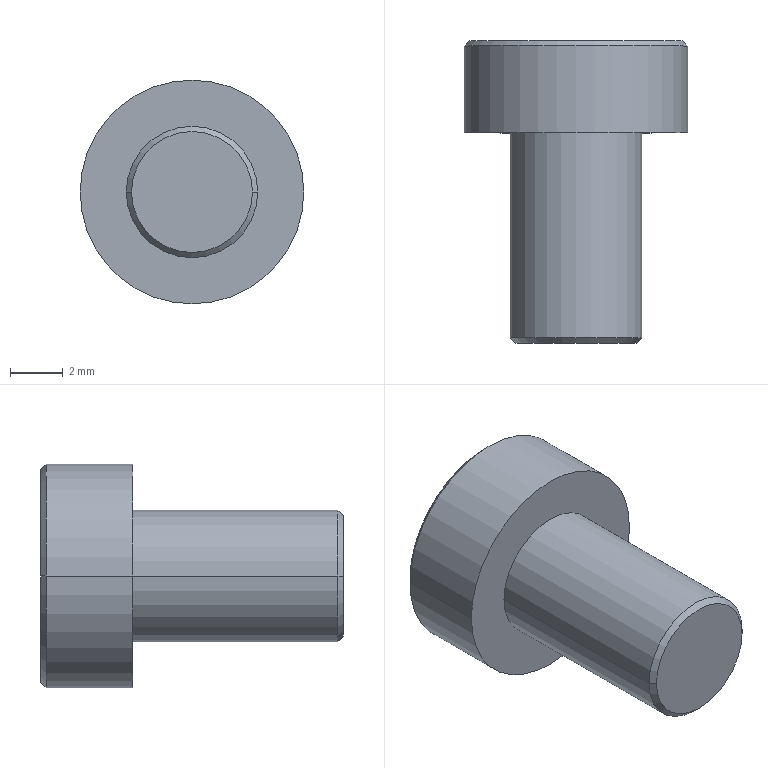Part | SolidWorks | features Chamfer 1, ICE 1, MoveCopyBody 1, Revolution 1 | 1 solid | 25 faces | box 8.5 x 11.5 x 8.5 mm | volume 331.771 mm3 | plane 15 | cone 6 | cylinder 4 | commonest cylinder face diameters 5 x2 8.5 x2
STEP:
#1=CARTESIAN_POINT('',(0.,6.434,0.));
#2=VERTEX_POINT('',#1);
#3=CARTESIAN_POINT('',(1.5,7.3,0.));
#4=VERTEX_POINT('',#3);
#5=CARTESIAN_POINT('',(0.,6.434,0.));
#6=DIRECTION('',(0.866,0.5,0.));
#7=VECTOR('',#6,1000.);
#8=LINE('',#5,#7);
#9=EDGE_CURVE('',#2,#4,#8,.T.);
#10=ORIENTED_EDGE('',*,*,#9,.F.);
#11=CARTESIAN_POINT('',(-1.5,7.3,0.));
#12=VERTEX_POINT('',#11);
#13=CARTESIAN_POINT('',(0.,6.434,0.));
#14=DIRECTION('',(-0.866,0.5,0.));
#15=VECTOR('',#14,1000.);
#16=LINE('',#13,#15);
#17=EDGE_CURVE('',#2,#12,#16,.T.);
#18=ORIENTED_EDGE('',*,*,#17,.T.);
#19=CARTESIAN_POINT('',(-1.299,7.3,0.75));
#20=VERTEX_POINT('',#19);
#21=CARTESIAN_POINT('',(0.,7.3,0.));
#22=DIRECTION('',(0.,1.,0.));
#23=DIRECTION('',(1.,0.,0.));
#24=AXIS2_PLACEMENT_3D('',#21,#22,#23);
#25=CIRCLE('',#24,1.5);
#26=EDGE_CURVE('',#12,#20,#25,.T.);
#27=ORIENTED_EDGE('',*,*,#26,.T.);
#28=CARTESIAN_POINT('',(0.,7.3,1.5));
#29=VERTEX_POINT('',#28);
#30=CARTESIAN_POINT('',(0.,7.3,0.));
#31=DIRECTION('',(0.,1.,0.));
#32=DIRECTION('',(1.,0.,0.));
#33=AXIS2_PLACEMENT_3D('',#30,#31,#32);
#34=CIRCLE('',#33,1.5);
#35=EDGE_CURVE('',#20,#29,#34,.T.);
#36=ORIENTED_EDGE('',*,*,#35,.T.);
#37=CARTESIAN_POINT('',(1.299,7.3,0.75));
#38=VERTEX_POINT('',#37);
#39=CARTESIAN_POINT('',(0.,7.3,0.));
#40=DIRECTION('',(0.,1.,0.));
#41=DIRECTION('',(1.,0.,0.));
#42=AXIS2_PLACEMENT_3D('',#39,#40,#41);
#43=CIRCLE('',#42,1.5);
#44=EDGE_CURVE('',#29,#38,#43,.T.);
#45=ORIENTED_EDGE('',*,*,#44,.T.);
#46=CARTESIAN_POINT('',(0.,7.3,0.));
#47=DIRECTION('',(0.,1.,0.));
#48=DIRECTION('',(1.,0.,0.));
#49=AXIS2_PLACEMENT_3D('',#46,#47,#48);
#50=CIRCLE('',#49,1.5);
#51=EDGE_CURVE('',#38,#4,#50,.T.);
#52=ORIENTED_EDGE('',*,*,#51,.T.);
#53=EDGE_LOOP('',(#10,#18,#27,#36,#45,#52));
#54=FACE_OUTER_BOUND('',#53,.T.);
#55=CARTESIAN_POINT('',(0.,1006.434,0.));
#56=DIRECTION('',(0.,1.,0.));
#57=DIRECTION('',(1.,0.,0.));
#58=AXIS2_PLACEMENT_3D('',#55,#56,#57);
#59=CONICAL_SURFACE('',#58,1732.051,1.047);
#60=ADVANCED_FACE('',(#54),#59,.F.);
#61=CARTESIAN_POINT('',(-2.3,-1.5,0.));
#62=VERTEX_POINT('',#61);
#63=CARTESIAN_POINT('',(2.3,-1.5,0.));
#64=VERTEX_POINT('',#63);
#65=CARTESIAN_POINT('',(0.,-1.5,0.));
#66=DIRECTION('',(0.,-1.,0.));
#67=DIRECTION('',(-1.,0.,0.));
#68=AXIS2_PLACEMENT_3D('',#65,#66,#67);
#69=CIRCLE('',#68,2.3);
#70=EDGE_CURVE('',#62,#64,#69,.T.);
#71=ORIENTED_EDGE('',*,*,#70,.F.);
#72=CARTESIAN_POINT('',(-2.5,-1.3,0.));
#73=VERTEX_POINT('',#72);
#74=CARTESIAN_POINT('',(-2.5,-1.3,0.));
#75=DIRECTION('',(-0.7071,0.7071,0.));
#76=VECTOR('',#75,1000.);
#77=LINE('',#74,#76);
#78=EDGE_CURVE('',#62,#73,#77,.T.);
#79=ORIENTED_EDGE('',*,*,#78,.T.);
#80=CARTESIAN_POINT('',(2.5,-1.3,0.));
#81=VERTEX_POINT('',#80);
#82=CARTESIAN_POINT('',(0.,-1.3,0.));
#83=DIRECTION('',(0.,1.,0.));
#84=DIRECTION('',(-1.,0.,0.));
#85=AXIS2_PLACEMENT_3D('',#82,#83,#84);
#86=CIRCLE('',#85,2.5);
#87=EDGE_CURVE('',#81,#73,#86,.T.);
#88=ORIENTED_EDGE('',*,*,#87,.F.);
#89=CARTESIAN_POINT('',(2.5,-1.3,0.));
#90=DIRECTION('',(0.7071,0.7071,0.));
#91=VECTOR('',#90,1000.);
#92=LINE('',#89,#91);
#93=EDGE_CURVE('',#64,#81,#92,.T.);
#94=ORIENTED_EDGE('',*,*,#93,.F.);
#95=EDGE_LOOP('',(#71,#79,#88,#94));
#96=FACE_OUTER_BOUND('',#95,.T.);
#97=CARTESIAN_POINT('',(0.,-1.3,0.));
#98=DIRECTION('',(0.,1.,0.));
#99=DIRECTION('',(1.,0.,0.));
#100=AXIS2_PLACEMENT_3D('',#97,#98,#99);
#101=CONICAL_SURFACE('',#100,2.5,0.7854);
#102=ADVANCED_FACE('',(#96),#101,.T.);
#103=CARTESIAN_POINT('',(4.05,10.,0.));
#104=VERTEX_POINT('',#103);
#105=CARTESIAN_POINT('',(-4.05,10.,0.));
#106=VERTEX_POINT('',#105);
#107=CARTESIAN_POINT('',(0.,10.,0.));
#108=DIRECTION('',(0.,1.,0.));
#109=DIRECTION('',(1.,0.,0.));
#110=AXIS2_PLACEMENT_3D('',#107,#108,#109);
#111=CIRCLE('',#110,4.05);
#112=EDGE_CURVE('',#104,#106,#111,.T.);
#113=ORIENTED_EDGE('',*,*,#112,.F.);
#114=CARTESIAN_POINT('',(4.25,9.8,0.));
#115=VERTEX_POINT('',#114);
#116=CARTESIAN_POINT('',(4.05,10.,0.));
#117=DIRECTION('',(0.7071,-0.7071,0.));
#118=VECTOR('',#117,1000.);
#119=LINE('',#116,#118);
#120=EDGE_CURVE('',#104,#115,#119,.T.);
#121=ORIENTED_EDGE('',*,*,#120,.T.);
#122=CARTESIAN_POINT('',(-4.25,9.8,0.));
#123=VERTEX_POINT('',#122);
#124=CARTESIAN_POINT('',(0.,9.8,0.));
#125=DIRECTION('',(0.,-1.,0.));
#126=DIRECTION('',(1.,0.,0.));
#127=AXIS2_PLACEMENT_3D('',#124,#125,#126);
#128=CIRCLE('',#127,4.25);
#129=EDGE_CURVE('',#123,#115,#128,.T.);
#130=ORIENTED_EDGE('',*,*,#129,.F.);
#131=CARTESIAN_POINT('',(-4.05,10.,0.));
#132=DIRECTION('',(-0.7071,-0.7071,0.));
#133=VECTOR('',#132,1000.);
#134=LINE('',#131,#133);
#135=EDGE_CURVE('',#106,#123,#134,.T.);
#136=ORIENTED_EDGE('',*,*,#135,.F.);
#137=EDGE_LOOP('',(#113,#121,#130,#136));
#138=FACE_OUTER_BOUND('',#137,.T.);
#139=CARTESIAN_POINT('',(0.,10.,0.));
#140=DIRECTION('',(0.,-1.,0.));
#141=DIRECTION('',(-1.,0.,0.));
#142=AXIS2_PLACEMENT_3D('',#139,#140,#141);
#143=CONICAL_SURFACE('',#142,4.05,0.7854);
#144=ADVANCED_FACE('',(#138),#143,.T.);
#145=CARTESIAN_POINT('',(4.25,6.5,0.));
#146=VERTEX_POINT('',#145);
#147=CARTESIAN_POINT('',(-4.25,6.5,0.));
#148=VERTEX_POINT('',#147);
#149=CARTESIAN_POINT('',(0.,6.5,0.));
#150=DIRECTION('',(0.,1.,0.));
#151=DIRECTION('',(1.,0.,0.));
#152=AXIS2_PLACEMENT_3D('',#149,#150,#151);
#153=CIRCLE('',#152,4.25);
#154=EDGE_CURVE('',#146,#148,#153,.T.);
#155=ORIENTED_EDGE('',*,*,#154,.T.);
#156=CARTESIAN_POINT('',(-4.25,6.434,0.));
#157=DIRECTION('',(0.,1.,0.));
#158=VECTOR('',#157,1000.);
#159=LINE('',#156,#158);
#160=EDGE_CURVE('',#148,#123,#159,.T.);
#161=ORIENTED_EDGE('',*,*,#160,.T.);
#162=ORIENTED_EDGE('',*,*,#129,.T.);
#163=CARTESIAN_POINT('',(4.25,6.434,0.));
#164=DIRECTION('',(0.,1.,0.));
#165=VECTOR('',#164,1000.);
#166=LINE('',#163,#165);
#167=EDGE_CURVE('',#146,#115,#166,.T.);
#168=ORIENTED_EDGE('',*,*,#167,.F.);
#169=EDGE_LOOP('',(#155,#161,#162,#168));
#170=FACE_OUTER_BOUND('',#169,.T.);
#171=CARTESIAN_POINT('',(0.,6.434,0.));
#172=DIRECTION('',(0.,1.,0.));
#173=DIRECTION('',(1.,0.,0.));
#174=AXIS2_PLACEMENT_3D('',#171,#172,#173);
#175=CYLINDRICAL_SURFACE('',#174,4.25);
#176=ADVANCED_FACE('',(#170),#175,.T.);
#177=ORIENTED_EDGE('',*,*,#87,.T.);
#178=CARTESIAN_POINT('',(-2.5,6.5,0.));
#179=VERTEX_POINT('',#178);
#180=CARTESIAN_POINT('',(-2.5,6.434,0.));
#181=DIRECTION('',(0.,1.,0.));
#182=VECTOR('',#181,1000.);
#183=LINE('',#180,#182);
#184=EDGE_CURVE('',#73,#179,#183,.T.);
#185=ORIENTED_EDGE('',*,*,#184,.T.);
#186=CARTESIAN_POINT('',(2.5,6.5,0.));
#187=VERTEX_POINT('',#186);
#188=CARTESIAN_POINT('',(0.,6.5,0.));
#189=DIRECTION('',(0.,1.,0.));
#190=DIRECTION('',(1.,0.,0.));
#191=AXIS2_PLACEMENT_3D('',#188,#189,#190);
#192=CIRCLE('',#191,2.5);
#193=EDGE_CURVE('',#187,#179,#192,.T.);
#194=ORIENTED_EDGE('',*,*,#193,.F.);
#195=CARTESIAN_POINT('',(2.5,6.434,0.));
#196=DIRECTION('',(0.,1.,0.));
#197=VECTOR('',#196,1000.);
#198=LINE('',#195,#197);
#199=EDGE_CURVE('',#81,#187,#198,.T.);
#200=ORIENTED_EDGE('',*,*,#199,.F.);
#201=EDGE_LOOP('',(#177,#185,#194,#200));
#202=FACE_OUTER_BOUND('',#201,.T.);
#203=CARTESIAN_POINT('',(0.,6.434,0.));
#204=DIRECTION('',(0.,1.,0.));
#205=DIRECTION('',(1.,0.,0.));
#206=AXIS2_PLACEMENT_3D('',#203,#204,#205);
#207=CYLINDRICAL_SURFACE('',#206,2.5);
#208=ADVANCED_FACE('',(#202),#207,.T.);
#209=CARTESIAN_POINT('',(0.866,10.,1.5));
#210=VERTEX_POINT('',#209);
#211=CARTESIAN_POINT('',(1.732,10.,0.));
#212=VERTEX_POINT('',#211);
#213=CARTESIAN_POINT('',(0.866,10.,1.5));
#214=DIRECTION('',(0.5,0.,-0.866));
#215=VECTOR('',#214,1000.);
#216=LINE('',#213,#215);
#217=EDGE_CURVE('',#210,#212,#216,.T.);
#218=ORIENTED_EDGE('',*,*,#217,.F.);
#219=CARTESIAN_POINT('',(-0.866,10.,1.5));
#220=VERTEX_POINT('',#219);
#221=CARTESIAN_POINT('',(-0.866,10.,1.5));
#222=DIRECTION('',(1.,0.,0.));
#223=VECTOR('',#222,1000.);
#224=LINE('',#221,#223);
#225=EDGE_CURVE('',#220,#210,#224,.T.);
#226=ORIENTED_EDGE('',*,*,#225,.F.);
#227=CARTESIAN_POINT('',(-1.732,10.,0.));
#228=VERTEX_POINT('',#227);
#229=CARTESIAN_POINT('',(-1.732,10.,0.));
#230=DIRECTION('',(0.5,0.,0.866));
#231=VECTOR('',#230,1000.);
#232=LINE('',#229,#231);
#233=EDGE_CURVE('',#228,#220,#232,.T.);
#234=ORIENTED_EDGE('',*,*,#233,.F.);
#235=CARTESIAN_POINT('',(-0.866,10.,-1.5));
#236=VERTEX_POINT('',#235);
#237=CARTESIAN_POINT('',(-0.866,10.,-1.5));
#238=DIRECTION('',(-0.5,0.,0.866));
#239=VECTOR('',#238,1000.);
#240=LINE('',#237,#239);
#241=EDGE_CURVE('',#236,#228,#240,.T.);
#242=ORIENTED_EDGE('',*,*,#241,.F.);
#243=CARTESIAN_POINT('',(0.866,10.,-1.5));
#244=VERTEX_POINT('',#243);
#245=CARTESIAN_POINT('',(0.866,10.,-1.5));
#246=DIRECTION('',(-1.,0.,0.));
#247=VECTOR('',#246,1000.);
#248=LINE('',#245,#247);
#249=EDGE_CURVE('',#244,#236,#248,.T.);
#250=ORIENTED_EDGE('',*,*,#249,.F.);
#251=CARTESIAN_POINT('',(1.732,10.,0.));
#252=DIRECTION('',(-0.5,0.,-0.866));
#253=VECTOR('',#252,1000.);
#254=LINE('',#251,#253);
#255=EDGE_CURVE('',#212,#244,#254,.T.);
#256=ORIENTED_EDGE('',*,*,#255,.F.);
#257=EDGE_LOOP('',(#218,#226,#234,#242,#250,#256));
#258=FACE_BOUND('',#257,.T.);
#259=CARTESIAN_POINT('',(0.,10.,0.));
#260=DIRECTION('',(0.,1.,0.));
#261=DIRECTION('',(1.,0.,0.));
#262=AXIS2_PLACEMENT_3D('',#259,#260,#261);
#263=CIRCLE('',#262,4.05);
#264=EDGE_CURVE('',#106,#104,#263,.T.);
#265=ORIENTED_EDGE('',*,*,#264,.T.);
#266=ORIENTED_EDGE('',*,*,#112,.T.);
#267=EDGE_LOOP('',(#265,#266));
#268=FACE_OUTER_BOUND('',#267,.T.);
#269=CARTESIAN_POINT('',(-4.25,10.,0.));
#270=DIRECTION('',(0.,1.,0.));
#271=DIRECTION('',(1.,0.,0.));
#272=AXIS2_PLACEMENT_3D('',#269,#270,#271);
#273=PLANE('',#272);
#274=ADVANCED_FACE('',(#258,#268),#273,.T.);
#275=CARTESIAN_POINT('',(0.,-1.5,0.));
#276=DIRECTION('',(0.,-1.,0.));
#277=DIRECTION('',(-1.,0.,0.));
#278=AXIS2_PLACEMENT_3D('',#275,#276,#277);
#279=CIRCLE('',#278,2.3);
#280=EDGE_CURVE('',#64,#62,#279,.T.);
#281=ORIENTED_EDGE('',*,*,#280,.T.);
#282=ORIENTED_EDGE('',*,*,#70,.T.);
#283=EDGE_LOOP('',(#281,#282));
#284=FACE_OUTER_BOUND('',#283,.T.);
#285=CARTESIAN_POINT('',(-2.5,-1.5,0.));
#286=DIRECTION('',(0.,-1.,0.));
#287=DIRECTION('',(-1.,0.,0.));
#288=AXIS2_PLACEMENT_3D('',#285,#286,#287);
#289=PLANE('',#288);
#290=ADVANCED_FACE('',(#284),#289,.T.);
#291=ORIENTED_EDGE('',*,*,#184,.F.);
#292=CARTESIAN_POINT('',(0.,-1.3,0.));
#293=DIRECTION('',(0.,1.,0.));
#294=DIRECTION('',(-1.,0.,0.));
#295=AXIS2_PLACEMENT_3D('',#292,#293,#294);
#296=CIRCLE('',#295,2.5);
#297=EDGE_CURVE('',#73,#81,#296,.T.);
#298=ORIENTED_EDGE('',*,*,#297,.T.);
#299=ORIENTED_EDGE('',*,*,#199,.T.);
#300=CARTESIAN_POINT('',(0.,6.5,0.));
#301=DIRECTION('',(0.,1.,0.));
#302=DIRECTION('',(1.,0.,0.));
#303=AXIS2_PLACEMENT_3D('',#300,#301,#302);
#304=CIRCLE('',#303,2.5);
#305=EDGE_CURVE('',#179,#187,#304,.T.);
#306=ORIENTED_EDGE('',*,*,#305,.F.);
#307=EDGE_LOOP('',(#291,#298,#299,#306));
#308=FACE_OUTER_BOUND('',#307,.T.);
#309=CARTESIAN_POINT('',(0.,6.434,0.));
#310=DIRECTION('',(0.,1.,0.));
#311=DIRECTION('',(1.,0.,0.));
#312=AXIS2_PLACEMENT_3D('',#309,#310,#311);
#313=CYLINDRICAL_SURFACE('',#312,2.5);
#314=ADVANCED_FACE('',(#308),#313,.T.);
#315=ORIENTED_EDGE('',*,*,#193,.T.);
#316=ORIENTED_EDGE('',*,*,#305,.T.);
#317=EDGE_LOOP('',(#315,#316));
#318=FACE_BOUND('',#317,.T.);
#319=ORIENTED_EDGE('',*,*,#154,.F.);
#320=CARTESIAN_POINT('',(0.,6.5,0.));
#321=DIRECTION('',(0.,1.,0.));
#322=DIRECTION('',(1.,0.,0.));
#323=AXIS2_PLACEMENT_3D('',#320,#321,#322);
#324=CIRCLE('',#323,4.25);
#325=EDGE_CURVE('',#148,#146,#324,.T.);
#326=ORIENTED_EDGE('',*,*,#325,.F.);
#327=EDGE_LOOP('',(#319,#326));
#328=FACE_OUTER_BOUND('',#327,.T.);
#329=CARTESIAN_POINT('',(-2.5,6.5,0.));
#330=DIRECTION('',(0.,-1.,0.));
#331=DIRECTION('',(-1.,0.,0.));
#332=AXIS2_PLACEMENT_3D('',#329,#330,#331);
#333=PLANE('',#332);
#334=ADVANCED_FACE('',(#318,#328),#333,.T.);
#335=ORIENTED_EDGE('',*,*,#160,.F.);
#336=ORIENTED_EDGE('',*,*,#325,.T.);
#337=ORIENTED_EDGE('',*,*,#167,.T.);
#338=CARTESIAN_POINT('',(0.,9.8,0.));
#339=DIRECTION('',(0.,-1.,0.));
#340=DIRECTION('',(1.,0.,0.));
#341=AXIS2_PLACEMENT_3D('',#338,#339,#340);
#342=CIRCLE('',#341,4.25);
#343=EDGE_CURVE('',#115,#123,#342,.T.);
#344=ORIENTED_EDGE('',*,*,#343,.T.);
#345=EDGE_LOOP('',(#335,#336,#337,#344));
#346=FACE_OUTER_BOUND('',#345,.T.);
#347=CARTESIAN_POINT('',(0.,6.434,0.));
#348=DIRECTION('',(0.,1.,0.));
#349=DIRECTION('',(1.,0.,0.));
#350=AXIS2_PLACEMENT_3D('',#347,#348,#349);
#351=CYLINDRICAL_SURFACE('',#350,4.25);
#352=ADVANCED_FACE('',(#346),#351,.T.);
#353=ORIENTED_EDGE('',*,*,#120,.F.);
#354=ORIENTED_EDGE('',*,*,#264,.F.);
#355=ORIENTED_EDGE('',*,*,#135,.T.);
#356=ORIENTED_EDGE('',*,*,#343,.F.);
#357=EDGE_LOOP('',(#353,#354,#355,#356));
#358=FACE_OUTER_BOUND('',#357,.T.);
#359=CARTESIAN_POINT('',(0.,10.,0.));
#360=DIRECTION('',(0.,-1.,0.));
#361=DIRECTION('',(-1.,0.,0.));
#362=AXIS2_PLACEMENT_3D('',#359,#360,#361);
#363=CONICAL_SURFACE('',#362,4.05,0.7854);
#364=ADVANCED_FACE('',(#358),#363,.T.);
#365=ORIENTED_EDGE('',*,*,#78,.F.);
#366=ORIENTED_EDGE('',*,*,#280,.F.);
#367=ORIENTED_EDGE('',*,*,#93,.T.);
#368=ORIENTED_EDGE('',*,*,#297,.F.);
#369=EDGE_LOOP('',(#365,#366,#367,#368));
#370=FACE_OUTER_BOUND('',#369,.T.);
#371=CARTESIAN_POINT('',(0.,-1.3,0.));
#372=DIRECTION('',(0.,1.,0.));
#373=DIRECTION('',(1.,0.,0.));
#374=AXIS2_PLACEMENT_3D('',#371,#372,#373);
#375=CONICAL_SURFACE('',#374,2.5,0.7854);
#376=ADVANCED_FACE('',(#370),#375,.T.);
#377=CARTESIAN_POINT('',(0.866,7.3,-1.5));
#378=VERTEX_POINT('',#377);
#379=CARTESIAN_POINT('',(0.,7.3,-1.5));
#380=VERTEX_POINT('',#379);
#381=CARTESIAN_POINT('',(0.866,7.3,-1.5));
#382=DIRECTION('',(-1.,0.,0.));
#383=VECTOR('',#382,1000.);
#384=LINE('',#381,#383);
#385=EDGE_CURVE('',#378,#380,#384,.T.);
#386=ORIENTED_EDGE('',*,*,#385,.F.);
#387=CARTESIAN_POINT('',(0.866,7.3,-1.5));
#388=DIRECTION('',(0.,1.,0.));
#389=VECTOR('',#388,1000.);
#390=LINE('',#387,#389);
#391=EDGE_CURVE('',#378,#244,#390,.T.);
#392=ORIENTED_EDGE('',*,*,#391,.T.);
#393=ORIENTED_EDGE('',*,*,#249,.T.);
#394=CARTESIAN_POINT('',(-0.866,7.3,-1.5));
#395=VERTEX_POINT('',#394);
#396=CARTESIAN_POINT('',(-0.866,7.3,-1.5));
#397=DIRECTION('',(0.,1.,0.));
#398=VECTOR('',#397,1000.);
#399=LINE('',#396,#398);
#400=EDGE_CURVE('',#395,#236,#399,.T.);
#401=ORIENTED_EDGE('',*,*,#400,.F.);
#402=CARTESIAN_POINT('',(0.866,7.3,-1.5));
#403=DIRECTION('',(-1.,0.,0.));
#404=VECTOR('',#403,1000.);
#405=LINE('',#402,#404);
#406=EDGE_CURVE('',#380,#395,#405,.T.);
#407=ORIENTED_EDGE('',*,*,#406,.F.);
#408=EDGE_LOOP('',(#386,#392,#393,#401,#407));
#409=FACE_OUTER_BOUND('',#408,.T.);
#410=CARTESIAN_POINT('',(0.866,7.3,-1.5));
#411=DIRECTION('',(0.,0.,-1.));
#412=DIRECTION('',(1.,0.,0.));
#413=AXIS2_PLACEMENT_3D('',#410,#411,#412);
#414=PLANE('',#413);
#415=ADVANCED_FACE('',(#409),#414,.F.);
#416=CARTESIAN_POINT('',(1.732,7.3,0.));
#417=VERTEX_POINT('',#416);
#418=CARTESIAN_POINT('',(1.299,7.3,-0.75));
#419=VERTEX_POINT('',#418);
#420=CARTESIAN_POINT('',(1.732,7.3,0.));
#421=DIRECTION('',(-0.5,0.,-0.866));
#422=VECTOR('',#421,1000.);
#423=LINE('',#420,#422);
#424=EDGE_CURVE('',#417,#419,#423,.T.);
#425=ORIENTED_EDGE('',*,*,#424,.F.);
#426=CARTESIAN_POINT('',(1.732,7.3,0.));
#427=DIRECTION('',(0.,1.,0.));
#428=VECTOR('',#427,1000.);
#429=LINE('',#426,#428);
#430=EDGE_CURVE('',#417,#212,#429,.T.);
#431=ORIENTED_EDGE('',*,*,#430,.T.);
#432=ORIENTED_EDGE('',*,*,#255,.T.);
#433=ORIENTED_EDGE('',*,*,#391,.F.);
#434=CARTESIAN_POINT('',(1.732,7.3,0.));
#435=DIRECTION('',(-0.5,0.,-0.866));
#436=VECTOR('',#435,1000.);
#437=LINE('',#434,#436);
#438=EDGE_CURVE('',#419,#378,#437,.T.);
#439=ORIENTED_EDGE('',*,*,#438,.F.);
#440=EDGE_LOOP('',(#425,#431,#432,#433,#439));
#441=FACE_OUTER_BOUND('',#440,.T.);
#442=CARTESIAN_POINT('',(1.732,7.3,0.));
#443=DIRECTION('',(0.866,0.,-0.5));
#444=DIRECTION('',(0.5,0.,0.866));
#445=AXIS2_PLACEMENT_3D('',#442,#443,#444);
#446=PLANE('',#445);
#447=ADVANCED_FACE('',(#441),#446,.F.);
#448=CARTESIAN_POINT('',(0.866,7.3,1.5));
#449=VERTEX_POINT('',#448);
#450=CARTESIAN_POINT('',(0.866,7.3,1.5));
#451=DIRECTION('',(0.5,0.,-0.866));
#452=VECTOR('',#451,1000.);
#453=LINE('',#450,#452);
#454=EDGE_CURVE('',#449,#38,#453,.T.);
#455=ORIENTED_EDGE('',*,*,#454,.F.);
#456=CARTESIAN_POINT('',(0.866,7.3,1.5));
#457=DIRECTION('',(0.,1.,0.));
#458=VECTOR('',#457,1000.);
#459=LINE('',#456,#458);
#460=EDGE_CURVE('',#449,#210,#459,.T.);
#461=ORIENTED_EDGE('',*,*,#460,.T.);
#462=ORIENTED_EDGE('',*,*,#217,.T.);
#463=ORIENTED_EDGE('',*,*,#430,.F.);
#464=CARTESIAN_POINT('',(0.866,7.3,1.5));
#465=DIRECTION('',(0.5,0.,-0.866));
#466=VECTOR('',#465,1000.);
#467=LINE('',#464,#466);
#468=EDGE_CURVE('',#38,#417,#467,.T.);
#469=ORIENTED_EDGE('',*,*,#468,.F.);
#470=EDGE_LOOP('',(#455,#461,#462,#463,#469));
#471=FACE_OUTER_BOUND('',#470,.T.);
#472=CARTESIAN_POINT('',(0.866,7.3,1.5));
#473=DIRECTION('',(0.866,0.,0.5));
#474=DIRECTION('',(-0.5,0.,0.866));
#475=AXIS2_PLACEMENT_3D('',#472,#473,#474);
#476=PLANE('',#475);
#477=ADVANCED_FACE('',(#471),#476,.F.);
#478=CARTESIAN_POINT('',(-0.866,7.3,1.5));
#479=VERTEX_POINT('',#478);
#480=CARTESIAN_POINT('',(-0.866,7.3,1.5));
#481=DIRECTION('',(1.,0.,0.));
#482=VECTOR('',#481,1000.);
#483=LINE('',#480,#482);
#484=EDGE_CURVE('',#479,#29,#483,.T.);
#485=ORIENTED_EDGE('',*,*,#484,.F.);
#486=CARTESIAN_POINT('',(-0.866,7.3,1.5));
#487=DIRECTION('',(0.,1.,0.));
#488=VECTOR('',#487,1000.);
#489=LINE('',#486,#488);
#490=EDGE_CURVE('',#479,#220,#489,.T.);
#491=ORIENTED_EDGE('',*,*,#490,.T.);
#492=ORIENTED_EDGE('',*,*,#225,.T.);
#493=ORIENTED_EDGE('',*,*,#460,.F.);
#494=CARTESIAN_POINT('',(-0.866,7.3,1.5));
#495=DIRECTION('',(1.,0.,0.));
#496=VECTOR('',#495,1000.);
#497=LINE('',#494,#496);
#498=EDGE_CURVE('',#29,#449,#497,.T.);
#499=ORIENTED_EDGE('',*,*,#498,.F.);
#500=EDGE_LOOP('',(#485,#491,#492,#493,#499));
#501=FACE_OUTER_BOUND('',#500,.T.);
#502=CARTESIAN_POINT('',(-0.866,7.3,1.5));
#503=DIRECTION('',(0.,0.,1.));
#504=DIRECTION('',(-1.,0.,0.));
#505=AXIS2_PLACEMENT_3D('',#502,#503,#504);
#506=PLANE('',#505);
#507=ADVANCED_FACE('',(#501),#506,.F.);
#508=CARTESIAN_POINT('',(-1.732,7.3,0.));
#509=VERTEX_POINT('',#508);
#510=CARTESIAN_POINT('',(-1.732,7.3,0.));
#511=DIRECTION('',(0.5,0.,0.866));
#512=VECTOR('',#511,1000.);
#513=LINE('',#510,#512);
#514=EDGE_CURVE('',#509,#20,#513,.T.);
#515=ORIENTED_EDGE('',*,*,#514,.F.);
#516=CARTESIAN_POINT('',(-1.732,7.3,0.));
#517=DIRECTION('',(0.,1.,0.));
#518=VECTOR('',#517,1000.);
#519=LINE('',#516,#518);
#520=EDGE_CURVE('',#509,#228,#519,.T.);
#521=ORIENTED_EDGE('',*,*,#520,.T.);
#522=ORIENTED_EDGE('',*,*,#233,.T.);
#523=ORIENTED_EDGE('',*,*,#490,.F.);
#524=CARTESIAN_POINT('',(-1.732,7.3,0.));
#525=DIRECTION('',(0.5,0.,0.866));
#526=VECTOR('',#525,1000.);
#527=LINE('',#524,#526);
#528=EDGE_CURVE('',#20,#479,#527,.T.);
#529=ORIENTED_EDGE('',*,*,#528,.F.);
#530=EDGE_LOOP('',(#515,#521,#522,#523,#529));
#531=FACE_OUTER_BOUND('',#530,.T.);
#532=CARTESIAN_POINT('',(-1.732,7.3,0.));
#533=DIRECTION('',(-0.866,0.,0.5));
#534=DIRECTION('',(-0.5,0.,-0.866));
#535=AXIS2_PLACEMENT_3D('',#532,#533,#534);
#536=PLANE('',#535);
#537=ADVANCED_FACE('',(#531),#536,.F.);
#538=CARTESIAN_POINT('',(-1.299,7.3,-0.75));
#539=VERTEX_POINT('',#538);
#540=CARTESIAN_POINT('',(-0.866,7.3,-1.5));
#541=DIRECTION('',(-0.5,0.,0.866));
#542=VECTOR('',#541,1000.);
#543=LINE('',#540,#542);
#544=EDGE_CURVE('',#395,#539,#543,.T.);
#545=ORIENTED_EDGE('',*,*,#544,.F.);
#546=ORIENTED_EDGE('',*,*,#400,.T.);
#547=ORIENTED_EDGE('',*,*,#241,.T.);
#548=ORIENTED_EDGE('',*,*,#520,.F.);
#549=CARTESIAN_POINT('',(-0.866,7.3,-1.5));
#550=DIRECTION('',(-0.5,0.,0.866));
#551=VECTOR('',#550,1000.);
#552=LINE('',#549,#551);
#553=EDGE_CURVE('',#539,#509,#552,.T.);
#554=ORIENTED_EDGE('',*,*,#553,.F.);
#555=EDGE_LOOP('',(#545,#546,#547,#548,#554));
#556=FACE_OUTER_BOUND('',#555,.T.);
#557=CARTESIAN_POINT('',(-0.866,7.3,-1.5));
#558=DIRECTION('',(-0.866,0.,-0.5));
#559=DIRECTION('',(0.5,0.,-0.866));
#560=AXIS2_PLACEMENT_3D('',#557,#558,#559);
#561=PLANE('',#560);
#562=ADVANCED_FACE('',(#556),#561,.F.);
#563=ORIENTED_EDGE('',*,*,#498,.T.);
#564=ORIENTED_EDGE('',*,*,#454,.T.);
#565=ORIENTED_EDGE('',*,*,#44,.F.);
#566=EDGE_LOOP('',(#563,#564,#565));
#567=FACE_OUTER_BOUND('',#566,.T.);
#568=CARTESIAN_POINT('',(-0.866,7.3,-1.5));
#569=DIRECTION('',(0.,1.,0.));
#570=DIRECTION('',(0.,0.,1.));
#571=AXIS2_PLACEMENT_3D('',#568,#569,#570);
#572=PLANE('',#571);
#573=ADVANCED_FACE('',(#567),#572,.T.);
#574=ORIENTED_EDGE('',*,*,#468,.T.);
#575=ORIENTED_EDGE('',*,*,#424,.T.);
#576=CARTESIAN_POINT('',(0.,7.3,0.));
#577=DIRECTION('',(0.,1.,0.));
#578=DIRECTION('',(1.,0.,0.));
#579=AXIS2_PLACEMENT_3D('',#576,#577,#578);
#580=CIRCLE('',#579,1.5);
#581=EDGE_CURVE('',#4,#419,#580,.T.);
#582=ORIENTED_EDGE('',*,*,#581,.F.);
#583=ORIENTED_EDGE('',*,*,#51,.F.);
#584=EDGE_LOOP('',(#574,#575,#582,#583));
#585=FACE_OUTER_BOUND('',#584,.T.);
#586=CARTESIAN_POINT('',(-0.866,7.3,-1.5));
#587=DIRECTION('',(0.,1.,0.));
#588=DIRECTION('',(0.,0.,1.));
#589=AXIS2_PLACEMENT_3D('',#586,#587,#588);
#590=PLANE('',#589);
#591=ADVANCED_FACE('',(#585),#590,.T.);
#592=ORIENTED_EDGE('',*,*,#438,.T.);
#593=ORIENTED_EDGE('',*,*,#385,.T.);
#594=CARTESIAN_POINT('',(0.,7.3,0.));
#595=DIRECTION('',(0.,1.,0.));
#596=DIRECTION('',(1.,0.,0.));
#597=AXIS2_PLACEMENT_3D('',#594,#595,#596);
#598=CIRCLE('',#597,1.5);
#599=EDGE_CURVE('',#419,#380,#598,.T.);
#600=ORIENTED_EDGE('',*,*,#599,.F.);
#601=EDGE_LOOP('',(#592,#593,#600));
#602=FACE_OUTER_BOUND('',#601,.T.);
#603=CARTESIAN_POINT('',(-0.866,7.3,-1.5));
#604=DIRECTION('',(0.,1.,0.));
#605=DIRECTION('',(0.,0.,1.));
#606=AXIS2_PLACEMENT_3D('',#603,#604,#605);
#607=PLANE('',#606);
#608=ADVANCED_FACE('',(#602),#607,.T.);
#609=ORIENTED_EDGE('',*,*,#406,.T.);
#610=ORIENTED_EDGE('',*,*,#544,.T.);
#611=CARTESIAN_POINT('',(0.,7.3,0.));
#612=DIRECTION('',(0.,1.,0.));
#613=DIRECTION('',(1.,0.,0.));
#614=AXIS2_PLACEMENT_3D('',#611,#612,#613);
#615=CIRCLE('',#614,1.5);
#616=EDGE_CURVE('',#380,#539,#615,.T.);
#617=ORIENTED_EDGE('',*,*,#616,.F.);
#618=EDGE_LOOP('',(#609,#610,#617));
#619=FACE_OUTER_BOUND('',#618,.T.);
#620=CARTESIAN_POINT('',(-0.866,7.3,-1.5));
#621=DIRECTION('',(0.,1.,0.));
#622=DIRECTION('',(0.,0.,1.));
#623=AXIS2_PLACEMENT_3D('',#620,#621,#622);
#624=PLANE('',#623);
#625=ADVANCED_FACE('',(#619),#624,.T.);
#626=ORIENTED_EDGE('',*,*,#553,.T.);
#627=ORIENTED_EDGE('',*,*,#514,.T.);
#628=ORIENTED_EDGE('',*,*,#26,.F.);
#629=CARTESIAN_POINT('',(0.,7.3,0.));
#630=DIRECTION('',(0.,1.,0.));
#631=DIRECTION('',(1.,0.,0.));
#632=AXIS2_PLACEMENT_3D('',#629,#630,#631);
#633=CIRCLE('',#632,1.5);
#634=EDGE_CURVE('',#539,#12,#633,.T.);
#635=ORIENTED_EDGE('',*,*,#634,.F.);
#636=EDGE_LOOP('',(#626,#627,#628,#635));
#637=FACE_OUTER_BOUND('',#636,.T.);
#638=CARTESIAN_POINT('',(-0.866,7.3,-1.5));
#639=DIRECTION('',(0.,1.,0.));
#640=DIRECTION('',(0.,0.,1.));
#641=AXIS2_PLACEMENT_3D('',#638,#639,#640);
#642=PLANE('',#641);
#643=ADVANCED_FACE('',(#637),#642,.T.);
#644=ORIENTED_EDGE('',*,*,#528,.T.);
#645=ORIENTED_EDGE('',*,*,#484,.T.);
#646=ORIENTED_EDGE('',*,*,#35,.F.);
#647=EDGE_LOOP('',(#644,#645,#646));
#648=FACE_OUTER_BOUND('',#647,.T.);
#649=CARTESIAN_POINT('',(-0.866,7.3,-1.5));
#650=DIRECTION('',(0.,1.,0.));
#651=DIRECTION('',(0.,0.,1.));
#652=AXIS2_PLACEMENT_3D('',#649,#650,#651);
#653=PLANE('',#652);
#654=ADVANCED_FACE('',(#648),#653,.T.);
#655=ORIENTED_EDGE('',*,*,#17,.F.);
#656=ORIENTED_EDGE('',*,*,#9,.T.);
#657=ORIENTED_EDGE('',*,*,#581,.T.);
#658=ORIENTED_EDGE('',*,*,#599,.T.);
#659=ORIENTED_EDGE('',*,*,#616,.T.);
#660=ORIENTED_EDGE('',*,*,#634,.T.);
#661=EDGE_LOOP('',(#655,#656,#657,#658,#659,#660));
#662=FACE_OUTER_BOUND('',#661,.T.);
#663=CARTESIAN_POINT('',(0.,1006.434,0.));
#664=DIRECTION('',(0.,1.,0.));
#665=DIRECTION('',(1.,0.,0.));
#666=AXIS2_PLACEMENT_3D('',#663,#664,#665);
#667=CONICAL_SURFACE('',#666,1732.051,1.047);
#668=ADVANCED_FACE('',(#662),#667,.F.);
#669=CLOSED_SHELL('',(#60,#102,#144,#176,#208,#274,#290,#314,#334,#352,#364,#376,#415,#447,#477,#507,#537,#562,#573,#591,#608,#625,#643,#654,#668));
#670=MANIFOLD_SOLID_BREP('',#669);
#671=CARTESIAN_POINT('',(0.,0.,0.));
#672=DIRECTION('',(0.,0.,1.));
#673=DIRECTION('',(1.,0.,0.));
#674=AXIS2_PLACEMENT_3D('',#671,#672,#673);
#675=(LENGTH_UNIT()NAMED_UNIT(*)SI_UNIT(.MILLI.,.METRE.));
#676=UNCERTAINTY_MEASURE_WITH_UNIT(LENGTH_MEASURE(0.00001),#675,'','');
#677=(NAMED_UNIT(*)PLANE_ANGLE_UNIT()SI_UNIT($,.RADIAN.));
#678=(NAMED_UNIT(*)SI_UNIT($,.STERADIAN.)SOLID_ANGLE_UNIT());
#679=(GEOMETRIC_REPRESENTATION_CONTEXT(3)GLOBAL_UNCERTAINTY_ASSIGNED_CONTEXT((#676))GLOBAL_UNIT_ASSIGNED_CONTEXT((#675,#677,#678))REPRESENTATION_CONTEXT('',''));
#680=ADVANCED_BREP_SHAPE_REPRESENTATION('',(#670,#674),#679);